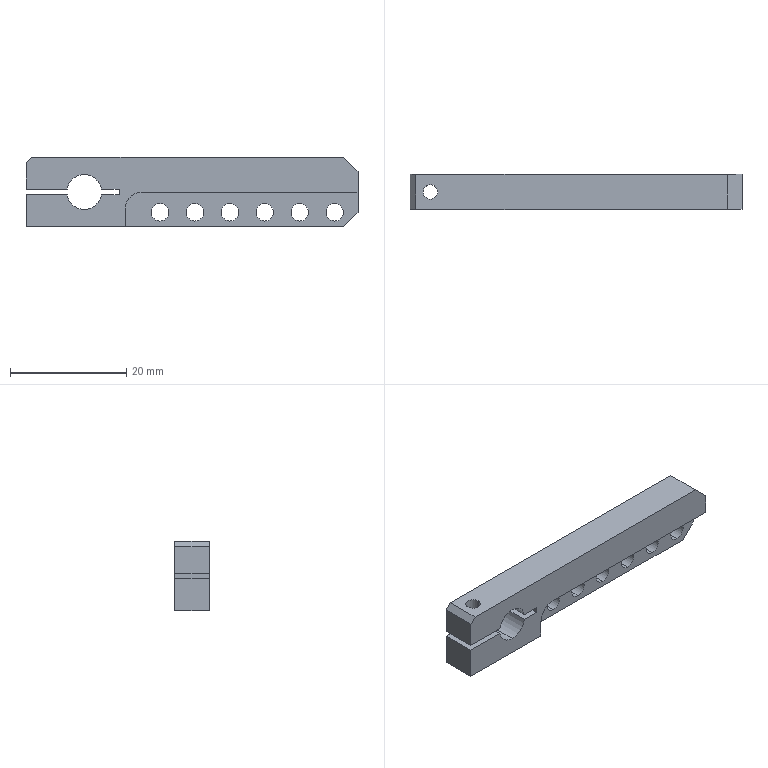Part | SolidWorks | features ICE 4, 3DProfileFeature 2, Chamfer 2, HoleWzd 2, Extrusion 1, Fillet 1, LPattern 1 | 1 solid | 38 faces | box 57 x 6 x 12 mm | volume 2922 mm3 | cylinder 20 | plane 18 | commonest cylinder face diameters 3 x12 6 x4 2.5 x2 3.5 x2
STEP:
#1=CARTESIAN_POINT('',(-9.5,6.,-2.));
#2=VERTEX_POINT('',#1);
#3=CARTESIAN_POINT('',(-9.5,6.,-5.));
#4=VERTEX_POINT('',#3);
#5=CARTESIAN_POINT('',(-9.5,6.,-3.5));
#6=DIRECTION('',(0.,-1.,0.));
#7=DIRECTION('',(0.,0.,-1.));
#8=AXIS2_PLACEMENT_3D('',#5,#6,#7);
#9=CIRCLE('',#8,1.5);
#10=EDGE_CURVE('',#2,#4,#9,.T.);
#11=ORIENTED_EDGE('',*,*,#10,.F.);
#12=CARTESIAN_POINT('',(-9.5,3.,-2.));
#13=VERTEX_POINT('',#12);
#14=CARTESIAN_POINT('',(-9.5,0.,-2.));
#15=DIRECTION('',(0.,-1.,0.));
#16=VECTOR('',#15,1000.);
#17=LINE('',#14,#16);
#18=EDGE_CURVE('',#2,#13,#17,.T.);
#19=ORIENTED_EDGE('',*,*,#18,.T.);
#20=CARTESIAN_POINT('',(-9.5,3.,-5.));
#21=VERTEX_POINT('',#20);
#22=CARTESIAN_POINT('',(-9.5,3.,-3.5));
#23=DIRECTION('',(0.,-1.,0.));
#24=DIRECTION('',(0.,0.,-1.));
#25=AXIS2_PLACEMENT_3D('',#22,#23,#24);
#26=CIRCLE('',#25,1.5);
#27=EDGE_CURVE('',#13,#21,#26,.T.);
#28=ORIENTED_EDGE('',*,*,#27,.T.);
#29=CARTESIAN_POINT('',(-9.5,0.,-5.));
#30=DIRECTION('',(0.,-1.,0.));
#31=VECTOR('',#30,1000.);
#32=LINE('',#29,#31);
#33=EDGE_CURVE('',#4,#21,#32,.T.);
#34=ORIENTED_EDGE('',*,*,#33,.F.);
#35=EDGE_LOOP('',(#11,#19,#28,#34));
#36=FACE_OUTER_BOUND('',#35,.T.);
#37=CARTESIAN_POINT('',(-9.5,0.,-3.5));
#38=DIRECTION('',(0.,-1.,0.));
#39=DIRECTION('',(0.,0.,-1.));
#40=AXIS2_PLACEMENT_3D('',#37,#38,#39);
#41=CYLINDRICAL_SURFACE('',#40,1.5);
#42=ADVANCED_FACE('',(#36),#41,.F.);
#43=CARTESIAN_POINT('',(-3.5,6.,-2.));
#44=VERTEX_POINT('',#43);
#45=CARTESIAN_POINT('',(-3.5,6.,-5.));
#46=VERTEX_POINT('',#45);
#47=CARTESIAN_POINT('',(-3.5,6.,-3.5));
#48=DIRECTION('',(0.,-1.,0.));
#49=DIRECTION('',(0.,0.,-1.));
#50=AXIS2_PLACEMENT_3D('',#47,#48,#49);
#51=CIRCLE('',#50,1.5);
#52=EDGE_CURVE('',#44,#46,#51,.T.);
#53=ORIENTED_EDGE('',*,*,#52,.F.);
#54=CARTESIAN_POINT('',(-3.5,3.,-2.));
#55=VERTEX_POINT('',#54);
#56=CARTESIAN_POINT('',(-3.5,0.,-2.));
#57=DIRECTION('',(0.,-1.,0.));
#58=VECTOR('',#57,1000.);
#59=LINE('',#56,#58);
#60=EDGE_CURVE('',#44,#55,#59,.T.);
#61=ORIENTED_EDGE('',*,*,#60,.T.);
#62=CARTESIAN_POINT('',(-3.5,3.,-5.));
#63=VERTEX_POINT('',#62);
#64=CARTESIAN_POINT('',(-3.5,3.,-3.5));
#65=DIRECTION('',(0.,-1.,0.));
#66=DIRECTION('',(0.,0.,-1.));
#67=AXIS2_PLACEMENT_3D('',#64,#65,#66);
#68=CIRCLE('',#67,1.5);
#69=EDGE_CURVE('',#55,#63,#68,.T.);
#70=ORIENTED_EDGE('',*,*,#69,.T.);
#71=CARTESIAN_POINT('',(-3.5,0.,-5.));
#72=DIRECTION('',(0.,-1.,0.));
#73=VECTOR('',#72,1000.);
#74=LINE('',#71,#73);
#75=EDGE_CURVE('',#46,#63,#74,.T.);
#76=ORIENTED_EDGE('',*,*,#75,.F.);
#77=EDGE_LOOP('',(#53,#61,#70,#76));
#78=FACE_OUTER_BOUND('',#77,.T.);
#79=CARTESIAN_POINT('',(-3.5,0.,-3.5));
#80=DIRECTION('',(0.,-1.,0.));
#81=DIRECTION('',(0.,0.,-1.));
#82=AXIS2_PLACEMENT_3D('',#79,#80,#81);
#83=CYLINDRICAL_SURFACE('',#82,1.5);
#84=ADVANCED_FACE('',(#78),#83,.F.);
#85=CARTESIAN_POINT('',(2.5,6.,-2.));
#86=VERTEX_POINT('',#85);
#87=CARTESIAN_POINT('',(2.5,6.,-5.));
#88=VERTEX_POINT('',#87);
#89=CARTESIAN_POINT('',(2.5,6.,-3.5));
#90=DIRECTION('',(0.,-1.,0.));
#91=DIRECTION('',(0.,0.,-1.));
#92=AXIS2_PLACEMENT_3D('',#89,#90,#91);
#93=CIRCLE('',#92,1.5);
#94=EDGE_CURVE('',#86,#88,#93,.T.);
#95=ORIENTED_EDGE('',*,*,#94,.F.);
#96=CARTESIAN_POINT('',(2.5,3.,-2.));
#97=VERTEX_POINT('',#96);
#98=CARTESIAN_POINT('',(2.5,0.,-2.));
#99=DIRECTION('',(0.,-1.,0.));
#100=VECTOR('',#99,1000.);
#101=LINE('',#98,#100);
#102=EDGE_CURVE('',#86,#97,#101,.T.);
#103=ORIENTED_EDGE('',*,*,#102,.T.);
#104=CARTESIAN_POINT('',(2.5,3.,-5.));
#105=VERTEX_POINT('',#104);
#106=CARTESIAN_POINT('',(2.5,3.,-3.5));
#107=DIRECTION('',(0.,-1.,0.));
#108=DIRECTION('',(0.,0.,-1.));
#109=AXIS2_PLACEMENT_3D('',#106,#107,#108);
#110=CIRCLE('',#109,1.5);
#111=EDGE_CURVE('',#97,#105,#110,.T.);
#112=ORIENTED_EDGE('',*,*,#111,.T.);
#113=CARTESIAN_POINT('',(2.5,0.,-5.));
#114=DIRECTION('',(0.,-1.,0.));
#115=VECTOR('',#114,1000.);
#116=LINE('',#113,#115);
#117=EDGE_CURVE('',#88,#105,#116,.T.);
#118=ORIENTED_EDGE('',*,*,#117,.F.);
#119=EDGE_LOOP('',(#95,#103,#112,#118));
#120=FACE_OUTER_BOUND('',#119,.T.);
#121=CARTESIAN_POINT('',(2.5,0.,-3.5));
#122=DIRECTION('',(0.,-1.,0.));
#123=DIRECTION('',(0.,0.,-1.));
#124=AXIS2_PLACEMENT_3D('',#121,#122,#123);
#125=CYLINDRICAL_SURFACE('',#124,1.5);
#126=ADVANCED_FACE('',(#120),#125,.F.);
#127=CARTESIAN_POINT('',(8.5,6.,-2.));
#128=VERTEX_POINT('',#127);
#129=CARTESIAN_POINT('',(8.5,6.,-5.));
#130=VERTEX_POINT('',#129);
#131=CARTESIAN_POINT('',(8.5,6.,-3.5));
#132=DIRECTION('',(0.,-1.,0.));
#133=DIRECTION('',(0.,0.,-1.));
#134=AXIS2_PLACEMENT_3D('',#131,#132,#133);
#135=CIRCLE('',#134,1.5);
#136=EDGE_CURVE('',#128,#130,#135,.T.);
#137=ORIENTED_EDGE('',*,*,#136,.F.);
#138=CARTESIAN_POINT('',(8.5,3.,-2.));
#139=VERTEX_POINT('',#138);
#140=CARTESIAN_POINT('',(8.5,0.,-2.));
#141=DIRECTION('',(0.,-1.,0.));
#142=VECTOR('',#141,1000.);
#143=LINE('',#140,#142);
#144=EDGE_CURVE('',#128,#139,#143,.T.);
#145=ORIENTED_EDGE('',*,*,#144,.T.);
#146=CARTESIAN_POINT('',(8.5,3.,-5.));
#147=VERTEX_POINT('',#146);
#148=CARTESIAN_POINT('',(8.5,3.,-3.5));
#149=DIRECTION('',(0.,-1.,0.));
#150=DIRECTION('',(0.,0.,-1.));
#151=AXIS2_PLACEMENT_3D('',#148,#149,#150);
#152=CIRCLE('',#151,1.5);
#153=EDGE_CURVE('',#139,#147,#152,.T.);
#154=ORIENTED_EDGE('',*,*,#153,.T.);
#155=CARTESIAN_POINT('',(8.5,0.,-5.));
#156=DIRECTION('',(0.,-1.,0.));
#157=VECTOR('',#156,1000.);
#158=LINE('',#155,#157);
#159=EDGE_CURVE('',#130,#147,#158,.T.);
#160=ORIENTED_EDGE('',*,*,#159,.F.);
#161=EDGE_LOOP('',(#137,#145,#154,#160));
#162=FACE_OUTER_BOUND('',#161,.T.);
#163=CARTESIAN_POINT('',(8.5,0.,-3.5));
#164=DIRECTION('',(0.,-1.,0.));
#165=DIRECTION('',(0.,0.,-1.));
#166=AXIS2_PLACEMENT_3D('',#163,#164,#165);
#167=CYLINDRICAL_SURFACE('',#166,1.5);
#168=ADVANCED_FACE('',(#162),#167,.F.);
#169=CARTESIAN_POINT('',(14.5,6.,-2.));
#170=VERTEX_POINT('',#169);
#171=CARTESIAN_POINT('',(14.5,6.,-5.));
#172=VERTEX_POINT('',#171);
#173=CARTESIAN_POINT('',(14.5,6.,-3.5));
#174=DIRECTION('',(0.,-1.,0.));
#175=DIRECTION('',(0.,0.,-1.));
#176=AXIS2_PLACEMENT_3D('',#173,#174,#175);
#177=CIRCLE('',#176,1.5);
#178=EDGE_CURVE('',#170,#172,#177,.T.);
#179=ORIENTED_EDGE('',*,*,#178,.F.);
#180=CARTESIAN_POINT('',(14.5,3.,-2.));
#181=VERTEX_POINT('',#180);
#182=CARTESIAN_POINT('',(14.5,0.,-2.));
#183=DIRECTION('',(0.,-1.,0.));
#184=VECTOR('',#183,1000.);
#185=LINE('',#182,#184);
#186=EDGE_CURVE('',#170,#181,#185,.T.);
#187=ORIENTED_EDGE('',*,*,#186,.T.);
#188=CARTESIAN_POINT('',(14.5,3.,-5.));
#189=VERTEX_POINT('',#188);
#190=CARTESIAN_POINT('',(14.5,3.,-3.5));
#191=DIRECTION('',(0.,-1.,0.));
#192=DIRECTION('',(0.,0.,-1.));
#193=AXIS2_PLACEMENT_3D('',#190,#191,#192);
#194=CIRCLE('',#193,1.5);
#195=EDGE_CURVE('',#181,#189,#194,.T.);
#196=ORIENTED_EDGE('',*,*,#195,.T.);
#197=CARTESIAN_POINT('',(14.5,0.,-5.));
#198=DIRECTION('',(0.,-1.,0.));
#199=VECTOR('',#198,1000.);
#200=LINE('',#197,#199);
#201=EDGE_CURVE('',#172,#189,#200,.T.);
#202=ORIENTED_EDGE('',*,*,#201,.F.);
#203=EDGE_LOOP('',(#179,#187,#196,#202));
#204=FACE_OUTER_BOUND('',#203,.T.);
#205=CARTESIAN_POINT('',(14.5,0.,-3.5));
#206=DIRECTION('',(0.,-1.,0.));
#207=DIRECTION('',(0.,0.,-1.));
#208=AXIS2_PLACEMENT_3D('',#205,#206,#207);
#209=CYLINDRICAL_SURFACE('',#208,1.5);
#210=ADVANCED_FACE('',(#204),#209,.F.);
#211=CARTESIAN_POINT('',(20.5,6.,-2.));
#212=VERTEX_POINT('',#211);
#213=CARTESIAN_POINT('',(20.5,6.,-5.));
#214=VERTEX_POINT('',#213);
#215=CARTESIAN_POINT('',(20.5,6.,-3.5));
#216=DIRECTION('',(0.,-1.,0.));
#217=DIRECTION('',(0.,0.,-1.));
#218=AXIS2_PLACEMENT_3D('',#215,#216,#217);
#219=CIRCLE('',#218,1.5);
#220=EDGE_CURVE('',#212,#214,#219,.T.);
#221=ORIENTED_EDGE('',*,*,#220,.F.);
#222=CARTESIAN_POINT('',(20.5,3.,-2.));
#223=VERTEX_POINT('',#222);
#224=CARTESIAN_POINT('',(20.5,0.,-2.));
#225=DIRECTION('',(0.,-1.,0.));
#226=VECTOR('',#225,1000.);
#227=LINE('',#224,#226);
#228=EDGE_CURVE('',#212,#223,#227,.T.);
#229=ORIENTED_EDGE('',*,*,#228,.T.);
#230=CARTESIAN_POINT('',(20.5,3.,-5.));
#231=VERTEX_POINT('',#230);
#232=CARTESIAN_POINT('',(20.5,3.,-3.5));
#233=DIRECTION('',(0.,-1.,0.));
#234=DIRECTION('',(0.,0.,-1.));
#235=AXIS2_PLACEMENT_3D('',#232,#233,#234);
#236=CIRCLE('',#235,1.5);
#237=EDGE_CURVE('',#223,#231,#236,.T.);
#238=ORIENTED_EDGE('',*,*,#237,.T.);
#239=CARTESIAN_POINT('',(20.5,0.,-5.));
#240=DIRECTION('',(0.,-1.,0.));
#241=VECTOR('',#240,1000.);
#242=LINE('',#239,#241);
#243=EDGE_CURVE('',#214,#231,#242,.T.);
#244=ORIENTED_EDGE('',*,*,#243,.F.);
#245=EDGE_LOOP('',(#221,#229,#238,#244));
#246=FACE_OUTER_BOUND('',#245,.T.);
#247=CARTESIAN_POINT('',(20.5,0.,-3.5));
#248=DIRECTION('',(0.,-1.,0.));
#249=DIRECTION('',(0.,0.,-1.));
#250=AXIS2_PLACEMENT_3D('',#247,#248,#249);
#251=CYLINDRICAL_SURFACE('',#250,1.5);
#252=ADVANCED_FACE('',(#246),#251,.F.);
#253=CARTESIAN_POINT('',(-27.75,3.,6.));
#254=VERTEX_POINT('',#253);
#255=CARTESIAN_POINT('',(-30.25,3.,6.));
#256=VERTEX_POINT('',#255);
#257=CARTESIAN_POINT('',(-29.,3.,6.));
#258=DIRECTION('',(0.,0.,-1.));
#259=DIRECTION('',(-1.,0.,0.));
#260=AXIS2_PLACEMENT_3D('',#257,#258,#259);
#261=CIRCLE('',#260,1.25);
#262=EDGE_CURVE('',#254,#256,#261,.T.);
#263=ORIENTED_EDGE('',*,*,#262,.F.);
#264=CARTESIAN_POINT('',(-27.75,3.,0.5));
#265=VERTEX_POINT('',#264);
#266=CARTESIAN_POINT('',(-27.75,3.,0.5));
#267=DIRECTION('',(0.,0.,-1.));
#268=VECTOR('',#267,1000.);
#269=LINE('',#266,#268);
#270=EDGE_CURVE('',#254,#265,#269,.T.);
#271=ORIENTED_EDGE('',*,*,#270,.T.);
#272=CARTESIAN_POINT('',(-30.25,3.,0.5));
#273=VERTEX_POINT('',#272);
#274=CARTESIAN_POINT('',(-29.,3.,0.5));
#275=DIRECTION('',(0.,0.,-1.));
#276=DIRECTION('',(-1.,0.,0.));
#277=AXIS2_PLACEMENT_3D('',#274,#275,#276);
#278=CIRCLE('',#277,1.25);
#279=EDGE_CURVE('',#265,#273,#278,.T.);
#280=ORIENTED_EDGE('',*,*,#279,.T.);
#281=CARTESIAN_POINT('',(-30.25,3.,0.5));
#282=DIRECTION('',(0.,0.,-1.));
#283=VECTOR('',#282,1000.);
#284=LINE('',#281,#283);
#285=EDGE_CURVE('',#256,#273,#284,.T.);
#286=ORIENTED_EDGE('',*,*,#285,.F.);
#287=EDGE_LOOP('',(#263,#271,#280,#286));
#288=FACE_OUTER_BOUND('',#287,.T.);
#289=CARTESIAN_POINT('',(-29.,3.,0.5));
#290=DIRECTION('',(0.,0.,-1.));
#291=DIRECTION('',(-1.,0.,0.));
#292=AXIS2_PLACEMENT_3D('',#289,#290,#291);
#293=CYLINDRICAL_SURFACE('',#292,1.25);
#294=ADVANCED_FACE('',(#288),#293,.F.);
#295=CARTESIAN_POINT('',(-27.25,3.,-0.5));
#296=VERTEX_POINT('',#295);
#297=CARTESIAN_POINT('',(-30.75,3.,-0.5));
#298=VERTEX_POINT('',#297);
#299=CARTESIAN_POINT('',(-29.,3.,-0.5));
#300=DIRECTION('',(0.,0.,-1.));
#301=DIRECTION('',(-1.,0.,0.));
#302=AXIS2_PLACEMENT_3D('',#299,#300,#301);
#303=CIRCLE('',#302,1.75);
#304=EDGE_CURVE('',#296,#298,#303,.T.);
#305=ORIENTED_EDGE('',*,*,#304,.F.);
#306=CARTESIAN_POINT('',(-27.25,3.,-6.));
#307=VERTEX_POINT('',#306);
#308=CARTESIAN_POINT('',(-27.25,3.,0.));
#309=DIRECTION('',(0.,0.,-1.));
#310=VECTOR('',#309,1000.);
#311=LINE('',#308,#310);
#312=EDGE_CURVE('',#296,#307,#311,.T.);
#313=ORIENTED_EDGE('',*,*,#312,.T.);
#314=CARTESIAN_POINT('',(-30.75,3.,-6.));
#315=VERTEX_POINT('',#314);
#316=CARTESIAN_POINT('',(-29.,3.,-6.));
#317=DIRECTION('',(0.,0.,-1.));
#318=DIRECTION('',(-1.,0.,0.));
#319=AXIS2_PLACEMENT_3D('',#316,#317,#318);
#320=CIRCLE('',#319,1.75);
#321=EDGE_CURVE('',#307,#315,#320,.T.);
#322=ORIENTED_EDGE('',*,*,#321,.T.);
#323=CARTESIAN_POINT('',(-30.75,3.,0.));
#324=DIRECTION('',(0.,0.,-1.));
#325=VECTOR('',#324,1000.);
#326=LINE('',#323,#325);
#327=EDGE_CURVE('',#298,#315,#326,.T.);
#328=ORIENTED_EDGE('',*,*,#327,.F.);
#329=EDGE_LOOP('',(#305,#313,#322,#328));
#330=FACE_OUTER_BOUND('',#329,.T.);
#331=CARTESIAN_POINT('',(-29.,3.,0.));
#332=DIRECTION('',(0.,0.,-1.));
#333=DIRECTION('',(-1.,0.,0.));
#334=AXIS2_PLACEMENT_3D('',#331,#332,#333);
#335=CYLINDRICAL_SURFACE('',#334,1.75);
#336=ADVANCED_FACE('',(#330),#335,.F.);
#337=CARTESIAN_POINT('',(-19.542,6.,-0.5));
#338=VERTEX_POINT('',#337);
#339=CARTESIAN_POINT('',(-22.5,6.,-3.));
#340=VERTEX_POINT('',#339);
#341=CARTESIAN_POINT('',(-22.5,6.,0.));
#342=DIRECTION('',(0.,1.,0.));
#343=DIRECTION('',(0.,0.,1.));
#344=AXIS2_PLACEMENT_3D('',#341,#342,#343);
#345=CIRCLE('',#344,3.);
#346=EDGE_CURVE('',#338,#340,#345,.T.);
#347=ORIENTED_EDGE('',*,*,#346,.T.);
#348=CARTESIAN_POINT('',(-22.5,0.,-3.));
#349=VERTEX_POINT('',#348);
#350=CARTESIAN_POINT('',(-22.5,6.,-3.));
#351=DIRECTION('',(0.,-1.,0.));
#352=VECTOR('',#351,1000.);
#353=LINE('',#350,#352);
#354=EDGE_CURVE('',#340,#349,#353,.T.);
#355=ORIENTED_EDGE('',*,*,#354,.T.);
#356=CARTESIAN_POINT('',(-19.542,0.,-0.5));
#357=VERTEX_POINT('',#356);
#358=CARTESIAN_POINT('',(-22.5,0.,0.));
#359=DIRECTION('',(0.,1.,0.));
#360=DIRECTION('',(0.,0.,1.));
#361=AXIS2_PLACEMENT_3D('',#358,#359,#360);
#362=CIRCLE('',#361,3.);
#363=EDGE_CURVE('',#357,#349,#362,.T.);
#364=ORIENTED_EDGE('',*,*,#363,.F.);
#365=CARTESIAN_POINT('',(-19.542,6.,-0.5));
#366=DIRECTION('',(0.,-1.,0.));
#367=VECTOR('',#366,1000.);
#368=LINE('',#365,#367);
#369=EDGE_CURVE('',#338,#357,#368,.T.);
#370=ORIENTED_EDGE('',*,*,#369,.F.);
#371=EDGE_LOOP('',(#347,#355,#364,#370));
#372=FACE_OUTER_BOUND('',#371,.T.);
#373=CARTESIAN_POINT('',(-22.5,6.,0.));
#374=DIRECTION('',(0.,-1.,0.));
#375=DIRECTION('',(0.,0.,-1.));
#376=AXIS2_PLACEMENT_3D('',#373,#374,#375);
#377=CYLINDRICAL_SURFACE('',#376,3.);
#378=ADVANCED_FACE('',(#372),#377,.F.);
#379=CARTESIAN_POINT('',(24.5,6.,-3.5));
#380=VERTEX_POINT('',#379);
#381=CARTESIAN_POINT('',(24.5,6.,3.5));
#382=VERTEX_POINT('',#381);
#383=CARTESIAN_POINT('',(24.5,6.,0.));
#384=DIRECTION('',(0.,0.,1.));
#385=VECTOR('',#384,1000.);
#386=LINE('',#383,#385);
#387=EDGE_CURVE('',#380,#382,#386,.T.);
#388=ORIENTED_EDGE('',*,*,#387,.F.);
#389=CARTESIAN_POINT('',(22.,6.,-6.));
#390=VERTEX_POINT('',#389);
#391=CARTESIAN_POINT('',(14.,6.,-14.));
#392=DIRECTION('',(-0.7071,0.,-0.7071));
#393=VECTOR('',#392,1000.);
#394=LINE('',#391,#393);
#395=EDGE_CURVE('',#380,#390,#394,.T.);
#396=ORIENTED_EDGE('',*,*,#395,.T.);
#397=CARTESIAN_POINT('',(-32.5,6.,-6.));
#398=VERTEX_POINT('',#397);
#399=CARTESIAN_POINT('',(-32.5,6.,-6.));
#400=DIRECTION('',(-1.,0.,0.));
#401=VECTOR('',#400,1000.);
#402=LINE('',#399,#401);
#403=EDGE_CURVE('',#390,#398,#402,.T.);
#404=ORIENTED_EDGE('',*,*,#403,.T.);
#405=CARTESIAN_POINT('',(-32.5,6.,-0.5));
#406=VERTEX_POINT('',#405);
#407=CARTESIAN_POINT('',(-32.5,6.,-6.));
#408=DIRECTION('',(0.,0.,1.));
#409=VECTOR('',#408,1000.);
#410=LINE('',#407,#409);
#411=EDGE_CURVE('',#398,#406,#410,.T.);
#412=ORIENTED_EDGE('',*,*,#411,.T.);
#413=CARTESIAN_POINT('',(-25.458,6.,-0.5));
#414=VERTEX_POINT('',#413);
#415=CARTESIAN_POINT('',(-48.5,6.,-0.5));
#416=DIRECTION('',(1.,0.,0.));
#417=VECTOR('',#416,1000.);
#418=LINE('',#415,#417);
#419=EDGE_CURVE('',#406,#414,#418,.T.);
#420=ORIENTED_EDGE('',*,*,#419,.T.);
#421=CARTESIAN_POINT('',(-22.5,6.,0.));
#422=DIRECTION('',(0.,1.,0.));
#423=DIRECTION('',(0.,0.,1.));
#424=AXIS2_PLACEMENT_3D('',#421,#422,#423);
#425=CIRCLE('',#424,3.);
#426=EDGE_CURVE('',#340,#414,#425,.T.);
#427=ORIENTED_EDGE('',*,*,#426,.F.);
#428=ORIENTED_EDGE('',*,*,#346,.F.);
#429=CARTESIAN_POINT('',(-16.5,6.,-0.5));
#430=VERTEX_POINT('',#429);
#431=CARTESIAN_POINT('',(-48.5,6.,-0.5));
#432=DIRECTION('',(1.,0.,0.));
#433=VECTOR('',#432,1000.);
#434=LINE('',#431,#433);
#435=EDGE_CURVE('',#338,#430,#434,.T.);
#436=ORIENTED_EDGE('',*,*,#435,.T.);
#437=CARTESIAN_POINT('',(-16.5,6.,0.5));
#438=VERTEX_POINT('',#437);
#439=CARTESIAN_POINT('',(-16.5,6.,0.5));
#440=DIRECTION('',(0.,0.,1.));
#441=VECTOR('',#440,1000.);
#442=LINE('',#439,#441);
#443=EDGE_CURVE('',#430,#438,#442,.T.);
#444=ORIENTED_EDGE('',*,*,#443,.T.);
#445=CARTESIAN_POINT('',(-19.542,6.,0.5));
#446=VERTEX_POINT('',#445);
#447=CARTESIAN_POINT('',(-48.5,6.,0.5));
#448=DIRECTION('',(-1.,0.,0.));
#449=VECTOR('',#448,1000.);
#450=LINE('',#447,#449);
#451=EDGE_CURVE('',#438,#446,#450,.T.);
#452=ORIENTED_EDGE('',*,*,#451,.T.);
#453=CARTESIAN_POINT('',(-25.458,6.,0.5));
#454=VERTEX_POINT('',#453);
#455=CARTESIAN_POINT('',(-22.5,6.,0.));
#456=DIRECTION('',(0.,1.,0.));
#457=DIRECTION('',(0.,0.,1.));
#458=AXIS2_PLACEMENT_3D('',#455,#456,#457);
#459=CIRCLE('',#458,3.);
#460=EDGE_CURVE('',#454,#446,#459,.T.);
#461=ORIENTED_EDGE('',*,*,#460,.F.);
#462=CARTESIAN_POINT('',(-32.5,6.,0.5));
#463=VERTEX_POINT('',#462);
#464=CARTESIAN_POINT('',(-48.5,6.,0.5));
#465=DIRECTION('',(-1.,0.,0.));
#466=VECTOR('',#465,1000.);
#467=LINE('',#464,#466);
#468=EDGE_CURVE('',#454,#463,#467,.T.);
#469=ORIENTED_EDGE('',*,*,#468,.T.);
#470=CARTESIAN_POINT('',(-32.5,6.,5.));
#471=VERTEX_POINT('',#470);
#472=CARTESIAN_POINT('',(-32.5,6.,-6.));
#473=DIRECTION('',(0.,0.,1.));
#474=VECTOR('',#473,1000.);
#475=LINE('',#472,#474);
#476=EDGE_CURVE('',#463,#471,#475,.T.);
#477=ORIENTED_EDGE('',*,*,#476,.T.);
#478=CARTESIAN_POINT('',(-31.5,6.,6.));
#479=VERTEX_POINT('',#478);
#480=CARTESIAN_POINT('',(-18.75,6.,18.75));
#481=DIRECTION('',(0.7071,0.,0.7071));
#482=VECTOR('',#481,1000.);
#483=LINE('',#480,#482);
#484=EDGE_CURVE('',#471,#479,#483,.T.);
#485=ORIENTED_EDGE('',*,*,#484,.T.);
#486=CARTESIAN_POINT('',(22.,6.,6.));
#487=VERTEX_POINT('',#486);
#488=CARTESIAN_POINT('',(-32.5,6.,6.));
#489=DIRECTION('',(1.,0.,0.));
#490=VECTOR('',#489,1000.);
#491=LINE('',#488,#490);
#492=EDGE_CURVE('',#479,#487,#491,.T.);
#493=ORIENTED_EDGE('',*,*,#492,.T.);
#494=CARTESIAN_POINT('',(14.,6.,14.));
#495=DIRECTION('',(0.7071,0.,-0.7071));
#496=VECTOR('',#495,1000.);
#497=LINE('',#494,#496);
#498=EDGE_CURVE('',#487,#382,#497,.T.);
#499=ORIENTED_EDGE('',*,*,#498,.T.);
#500=EDGE_LOOP('',(#388,#396,#404,#412,#420,#427,#428,#436,#444,#452,#461,#469,#477,#485,#493,#499));
#501=FACE_OUTER_BOUND('',#500,.T.);
#502=CARTESIAN_POINT('',(-3.5,6.,-3.5));
#503=DIRECTION('',(0.,-1.,0.));
#504=DIRECTION('',(0.,0.,-1.));
#505=AXIS2_PLACEMENT_3D('',#502,#503,#504);
#506=CIRCLE('',#505,1.5);
#507=EDGE_CURVE('',#46,#44,#506,.T.);
#508=ORIENTED_EDGE('',*,*,#507,.T.);
#509=ORIENTED_EDGE('',*,*,#52,.T.);
#510=EDGE_LOOP('',(#508,#509));
#511=FACE_BOUND('',#510,.T.);
#512=CARTESIAN_POINT('',(2.5,6.,-3.5));
#513=DIRECTION('',(0.,-1.,0.));
#514=DIRECTION('',(0.,0.,-1.));
#515=AXIS2_PLACEMENT_3D('',#512,#513,#514);
#516=CIRCLE('',#515,1.5);
#517=EDGE_CURVE('',#88,#86,#516,.T.);
#518=ORIENTED_EDGE('',*,*,#517,.T.);
#519=ORIENTED_EDGE('',*,*,#94,.T.);
#520=EDGE_LOOP('',(#518,#519));
#521=FACE_BOUND('',#520,.T.);
#522=CARTESIAN_POINT('',(8.5,6.,-3.5));
#523=DIRECTION('',(0.,-1.,0.));
#524=DIRECTION('',(0.,0.,-1.));
#525=AXIS2_PLACEMENT_3D('',#522,#523,#524);
#526=CIRCLE('',#525,1.5);
#527=EDGE_CURVE('',#130,#128,#526,.T.);
#528=ORIENTED_EDGE('',*,*,#527,.T.);
#529=ORIENTED_EDGE('',*,*,#136,.T.);
#530=EDGE_LOOP('',(#528,#529));
#531=FACE_BOUND('',#530,.T.);
#532=CARTESIAN_POINT('',(14.5,6.,-3.5));
#533=DIRECTION('',(0.,-1.,0.));
#534=DIRECTION('',(0.,0.,-1.));
#535=AXIS2_PLACEMENT_3D('',#532,#533,#534);
#536=CIRCLE('',#535,1.5);
#537=EDGE_CURVE('',#172,#170,#536,.T.);
#538=ORIENTED_EDGE('',*,*,#537,.T.);
#539=ORIENTED_EDGE('',*,*,#178,.T.);
#540=EDGE_LOOP('',(#538,#539));
#541=FACE_BOUND('',#540,.T.);
#542=CARTESIAN_POINT('',(20.5,6.,-3.5));
#543=DIRECTION('',(0.,-1.,0.));
#544=DIRECTION('',(0.,0.,-1.));
#545=AXIS2_PLACEMENT_3D('',#542,#543,#544);
#546=CIRCLE('',#545,1.5);
#547=EDGE_CURVE('',#214,#212,#546,.T.);
#548=ORIENTED_EDGE('',*,*,#547,.T.);
#549=ORIENTED_EDGE('',*,*,#220,.T.);
#550=EDGE_LOOP('',(#548,#549));
#551=FACE_BOUND('',#550,.T.);
#552=CARTESIAN_POINT('',(-9.5,6.,-3.5));
#553=DIRECTION('',(0.,-1.,0.));
#554=DIRECTION('',(0.,0.,-1.));
#555=AXIS2_PLACEMENT_3D('',#552,#553,#554);
#556=CIRCLE('',#555,1.5);
#557=EDGE_CURVE('',#4,#2,#556,.T.);
#558=ORIENTED_EDGE('',*,*,#557,.T.);
#559=ORIENTED_EDGE('',*,*,#10,.T.);
#560=EDGE_LOOP('',(#558,#559));
#561=FACE_BOUND('',#560,.T.);
#562=CARTESIAN_POINT('',(0.,6.,0.));
#563=DIRECTION('',(0.,1.,0.));
#564=DIRECTION('',(0.,0.,1.));
#565=AXIS2_PLACEMENT_3D('',#562,#563,#564);
#566=PLANE('',#565);
#567=ADVANCED_FACE('',(#501,#511,#521,#531,#541,#551,#561),#566,.T.);
#568=CARTESIAN_POINT('',(-32.5,0.,-6.));
#569=VERTEX_POINT('',#568);
#570=CARTESIAN_POINT('',(-32.5,0.,-0.5));
#571=VERTEX_POINT('',#570);
#572=CARTESIAN_POINT('',(-32.5,0.,-6.));
#573=DIRECTION('',(0.,0.,1.));
#574=VECTOR('',#573,1000.);
#575=LINE('',#572,#574);
#576=EDGE_CURVE('',#569,#571,#575,.T.);
#577=ORIENTED_EDGE('',*,*,#576,.T.);
#578=CARTESIAN_POINT('',(-32.5,6.,-0.5));
#579=DIRECTION('',(0.,1.,0.));
#580=VECTOR('',#579,1000.);
#581=LINE('',#578,#580);
#582=EDGE_CURVE('',#571,#406,#581,.T.);
#583=ORIENTED_EDGE('',*,*,#582,.T.);
#584=ORIENTED_EDGE('',*,*,#411,.F.);
#585=CARTESIAN_POINT('',(-32.5,6.,-6.));
#586=DIRECTION('',(0.,-1.,0.));
#587=VECTOR('',#586,1000.);
#588=LINE('',#585,#587);
#589=EDGE_CURVE('',#398,#569,#588,.T.);
#590=ORIENTED_EDGE('',*,*,#589,.T.);
#591=EDGE_LOOP('',(#577,#583,#584,#590));
#592=FACE_OUTER_BOUND('',#591,.T.);
#593=CARTESIAN_POINT('',(-32.5,6.,-6.));
#594=DIRECTION('',(1.,0.,0.));
#595=DIRECTION('',(0.,0.,-1.));
#596=AXIS2_PLACEMENT_3D('',#593,#594,#595);
#597=PLANE('',#596);
#598=ADVANCED_FACE('',(#592),#597,.F.);
#599=ORIENTED_EDGE('',*,*,#354,.F.);
#600=ORIENTED_EDGE('',*,*,#426,.T.);
#601=CARTESIAN_POINT('',(-25.458,0.,-0.5));
#602=VERTEX_POINT('',#601);
#603=CARTESIAN_POINT('',(-25.458,6.,-0.5));
#604=DIRECTION('',(0.,1.,0.));
#605=VECTOR('',#604,1000.);
#606=LINE('',#603,#605);
#607=EDGE_CURVE('',#602,#414,#606,.T.);
#608=ORIENTED_EDGE('',*,*,#607,.F.);
#609=CARTESIAN_POINT('',(-22.5,0.,0.));
#610=DIRECTION('',(0.,1.,0.));
#611=DIRECTION('',(0.,0.,1.));
#612=AXIS2_PLACEMENT_3D('',#609,#610,#611);
#613=CIRCLE('',#612,3.);
#614=EDGE_CURVE('',#349,#602,#613,.T.);
#615=ORIENTED_EDGE('',*,*,#614,.F.);
#616=EDGE_LOOP('',(#599,#600,#608,#615));
#617=FACE_OUTER_BOUND('',#616,.T.);
#618=CARTESIAN_POINT('',(-22.5,6.,0.));
#619=DIRECTION('',(0.,-1.,0.));
#620=DIRECTION('',(0.,0.,-1.));
#621=AXIS2_PLACEMENT_3D('',#618,#619,#620);
#622=CYLINDRICAL_SURFACE('',#621,3.);
#623=ADVANCED_FACE('',(#617),#622,.F.);
#624=CARTESIAN_POINT('',(24.5,0.,3.5));
#625=VERTEX_POINT('',#624);
#626=CARTESIAN_POINT('',(24.5,0.,0.));
#627=VERTEX_POINT('',#626);
#628=CARTESIAN_POINT('',(24.5,0.,6.));
#629=DIRECTION('',(0.,0.,-1.));
#630=VECTOR('',#629,1000.);
#631=LINE('',#628,#630);
#632=EDGE_CURVE('',#625,#627,#631,.T.);
#633=ORIENTED_EDGE('',*,*,#632,.F.);
#634=CARTESIAN_POINT('',(22.,0.,6.));
#635=VERTEX_POINT('',#634);
#636=CARTESIAN_POINT('',(24.5,0.,3.5));
#637=DIRECTION('',(-0.7071,0.,0.7071));
#638=VECTOR('',#637,1000.);
#639=LINE('',#636,#638);
#640=EDGE_CURVE('',#625,#635,#639,.T.);
#641=ORIENTED_EDGE('',*,*,#640,.T.);
#642=CARTESIAN_POINT('',(-31.5,0.,6.));
#643=VERTEX_POINT('',#642);
#644=CARTESIAN_POINT('',(-32.5,0.,6.));
#645=DIRECTION('',(1.,0.,0.));
#646=VECTOR('',#645,1000.);
#647=LINE('',#644,#646);
#648=EDGE_CURVE('',#643,#635,#647,.T.);
#649=ORIENTED_EDGE('',*,*,#648,.F.);
#650=CARTESIAN_POINT('',(-32.5,0.,5.));
#651=VERTEX_POINT('',#650);
#652=CARTESIAN_POINT('',(-31.5,0.,6.));
#653=DIRECTION('',(-0.7071,0.,-0.7071));
#654=VECTOR('',#653,1000.);
#655=LINE('',#652,#654);
#656=EDGE_CURVE('',#643,#651,#655,.T.);
#657=ORIENTED_EDGE('',*,*,#656,.T.);
#658=CARTESIAN_POINT('',(-32.5,0.,0.5));
#659=VERTEX_POINT('',#658);
#660=CARTESIAN_POINT('',(-32.5,0.,-6.));
#661=DIRECTION('',(0.,0.,1.));
#662=VECTOR('',#661,1000.);
#663=LINE('',#660,#662);
#664=EDGE_CURVE('',#659,#651,#663,.T.);
#665=ORIENTED_EDGE('',*,*,#664,.F.);
#666=CARTESIAN_POINT('',(-25.458,0.,0.5));
#667=VERTEX_POINT('',#666);
#668=CARTESIAN_POINT('',(-48.5,0.,0.5));
#669=DIRECTION('',(-1.,0.,0.));
#670=VECTOR('',#669,1000.);
#671=LINE('',#668,#670);
#672=EDGE_CURVE('',#667,#659,#671,.T.);
#673=ORIENTED_EDGE('',*,*,#672,.F.);
#674=CARTESIAN_POINT('',(-19.542,0.,0.5));
#675=VERTEX_POINT('',#674);
#676=CARTESIAN_POINT('',(-22.5,0.,0.));
#677=DIRECTION('',(0.,1.,0.));
#678=DIRECTION('',(0.,0.,1.));
#679=AXIS2_PLACEMENT_3D('',#676,#677,#678);
#680=CIRCLE('',#679,3.);
#681=EDGE_CURVE('',#667,#675,#680,.T.);
#682=ORIENTED_EDGE('',*,*,#681,.T.);
#683=CARTESIAN_POINT('',(-16.5,0.,0.5));
#684=VERTEX_POINT('',#683);
#685=CARTESIAN_POINT('',(-48.5,0.,0.5));
#686=DIRECTION('',(-1.,0.,0.));
#687=VECTOR('',#686,1000.);
#688=LINE('',#685,#687);
#689=EDGE_CURVE('',#684,#675,#688,.T.);
#690=ORIENTED_EDGE('',*,*,#689,.F.);
#691=CARTESIAN_POINT('',(-16.5,0.,-0.5));
#692=VERTEX_POINT('',#691);
#693=CARTESIAN_POINT('',(-16.5,0.,0.5));
#694=DIRECTION('',(0.,0.,1.));
#695=VECTOR('',#694,1000.);
#696=LINE('',#693,#695);
#697=EDGE_CURVE('',#692,#684,#696,.T.);
#698=ORIENTED_EDGE('',*,*,#697,.F.);
#699=CARTESIAN_POINT('',(-48.5,0.,-0.5));
#700=DIRECTION('',(1.,0.,0.));
#701=VECTOR('',#700,1000.);
#702=LINE('',#699,#701);
#703=EDGE_CURVE('',#357,#692,#702,.T.);
#704=ORIENTED_EDGE('',*,*,#703,.F.);
#705=ORIENTED_EDGE('',*,*,#363,.T.);
#706=ORIENTED_EDGE('',*,*,#614,.T.);
#707=CARTESIAN_POINT('',(-48.5,0.,-0.5));
#708=DIRECTION('',(1.,0.,0.));
#709=VECTOR('',#708,1000.);
#710=LINE('',#707,#709);
#711=EDGE_CURVE('',#571,#602,#710,.T.);
#712=ORIENTED_EDGE('',*,*,#711,.F.);
#713=ORIENTED_EDGE('',*,*,#576,.F.);
#714=CARTESIAN_POINT('',(-15.5,0.,-6.));
#715=VERTEX_POINT('',#714);
#716=CARTESIAN_POINT('',(-32.5,0.,-6.));
#717=DIRECTION('',(-1.,0.,0.));
#718=VECTOR('',#717,1000.);
#719=LINE('',#716,#718);
#720=EDGE_CURVE('',#715,#569,#719,.T.);
#721=ORIENTED_EDGE('',*,*,#720,.F.);
#722=CARTESIAN_POINT('',(-15.5,0.,-3.));
#723=VERTEX_POINT('',#722);
#724=CARTESIAN_POINT('',(-15.5,0.,-6.));
#725=DIRECTION('',(0.,0.,-1.));
#726=VECTOR('',#725,1000.);
#727=LINE('',#724,#726);
#728=EDGE_CURVE('',#723,#715,#727,.T.);
#729=ORIENTED_EDGE('',*,*,#728,.F.);
#730=CARTESIAN_POINT('',(-12.5,0.,0.));
#731=VERTEX_POINT('',#730);
#732=CARTESIAN_POINT('',(-12.5,0.,-3.));
#733=DIRECTION('',(0.,1.,0.));
#734=DIRECTION('',(0.,0.,1.));
#735=AXIS2_PLACEMENT_3D('',#732,#733,#734);
#736=CIRCLE('',#735,3.);
#737=EDGE_CURVE('',#723,#731,#736,.T.);
#738=ORIENTED_EDGE('',*,*,#737,.T.);
#739=CARTESIAN_POINT('',(32.5,0.,0.));
#740=DIRECTION('',(-1.,0.,0.));
#741=VECTOR('',#740,1000.);
#742=LINE('',#739,#741);
#743=EDGE_CURVE('',#627,#731,#742,.T.);
#744=ORIENTED_EDGE('',*,*,#743,.F.);
#745=EDGE_LOOP('',(#633,#641,#649,#657,#665,#673,#682,#690,#698,#704,#705,#706,#712,#713,#721,#729,#738,#744));
#746=FACE_OUTER_BOUND('',#745,.T.);
#747=CARTESIAN_POINT('',(0.,0.,0.));
#748=DIRECTION('',(0.,1.,0.));
#749=DIRECTION('',(0.,0.,1.));
#750=AXIS2_PLACEMENT_3D('',#747,#748,#749);
#751=PLANE('',#750);
#752=ADVANCED_FACE('',(#746),#751,.F.);
#753=CARTESIAN_POINT('',(-29.,3.,-6.));
#754=DIRECTION('',(0.,0.,-1.));
#755=DIRECTION('',(-1.,0.,0.));
#756=AXIS2_PLACEMENT_3D('',#753,#754,#755);
#757=CIRCLE('',#756,1.75);
#758=EDGE_CURVE('',#315,#307,#757,.T.);
#759=ORIENTED_EDGE('',*,*,#758,.F.);
#760=ORIENTED_EDGE('',*,*,#321,.F.);
#761=EDGE_LOOP('',(#759,#760));
#762=FACE_BOUND('',#761,.T.);
#763=ORIENTED_EDGE('',*,*,#403,.F.);
#764=CARTESIAN_POINT('',(22.,3.,-6.));
#765=VERTEX_POINT('',#764);
#766=CARTESIAN_POINT('',(22.,6.,-6.));
#767=DIRECTION('',(0.,-1.,0.));
#768=VECTOR('',#767,1000.);
#769=LINE('',#766,#768);
#770=EDGE_CURVE('',#390,#765,#769,.T.);
#771=ORIENTED_EDGE('',*,*,#770,.T.);
#772=CARTESIAN_POINT('',(-15.5,3.,-6.));
#773=VERTEX_POINT('',#772);
#774=CARTESIAN_POINT('',(32.5,3.,-6.));
#775=DIRECTION('',(1.,0.,0.));
#776=VECTOR('',#775,1000.);
#777=LINE('',#774,#776);
#778=EDGE_CURVE('',#773,#765,#777,.T.);
#779=ORIENTED_EDGE('',*,*,#778,.F.);
#780=CARTESIAN_POINT('',(-15.5,3.,-6.));
#781=DIRECTION('',(0.,-1.,0.));
#782=VECTOR('',#781,1000.);
#783=LINE('',#780,#782);
#784=EDGE_CURVE('',#773,#715,#783,.T.);
#785=ORIENTED_EDGE('',*,*,#784,.T.);
#786=ORIENTED_EDGE('',*,*,#720,.T.);
#787=ORIENTED_EDGE('',*,*,#589,.F.);
#788=EDGE_LOOP('',(#763,#771,#779,#785,#786,#787));
#789=FACE_OUTER_BOUND('',#788,.T.);
#790=CARTESIAN_POINT('',(-32.5,6.,-6.));
#791=DIRECTION('',(0.,0.,1.));
#792=DIRECTION('',(1.,0.,0.));
#793=AXIS2_PLACEMENT_3D('',#790,#791,#792);
#794=PLANE('',#793);
#795=ADVANCED_FACE('',(#762,#789),#794,.F.);
#796=ORIENTED_EDGE('',*,*,#664,.T.);
#797=CARTESIAN_POINT('',(-32.5,6.,5.));
#798=DIRECTION('',(0.,1.,0.));
#799=VECTOR('',#798,1000.);
#800=LINE('',#797,#799);
#801=EDGE_CURVE('',#651,#471,#800,.T.);
#802=ORIENTED_EDGE('',*,*,#801,.T.);
#803=ORIENTED_EDGE('',*,*,#476,.F.);
#804=CARTESIAN_POINT('',(-32.5,6.,0.5));
#805=DIRECTION('',(0.,-1.,0.));
#806=VECTOR('',#805,1000.);
#807=LINE('',#804,#806);
#808=EDGE_CURVE('',#463,#659,#807,.T.);
#809=ORIENTED_EDGE('',*,*,#808,.T.);
#810=EDGE_LOOP('',(#796,#802,#803,#809));
#811=FACE_OUTER_BOUND('',#810,.T.);
#812=CARTESIAN_POINT('',(-32.5,6.,-6.));
#813=DIRECTION('',(1.,0.,0.));
#814=DIRECTION('',(0.,0.,-1.));
#815=AXIS2_PLACEMENT_3D('',#812,#813,#814);
#816=PLANE('',#815);
#817=ADVANCED_FACE('',(#811),#816,.F.);
#818=CARTESIAN_POINT('',(-29.,3.,6.));
#819=DIRECTION('',(0.,0.,-1.));
#820=DIRECTION('',(-1.,0.,0.));
#821=AXIS2_PLACEMENT_3D('',#818,#819,#820);
#822=CIRCLE('',#821,1.25);
#823=EDGE_CURVE('',#256,#254,#822,.T.);
#824=ORIENTED_EDGE('',*,*,#823,.T.);
#825=ORIENTED_EDGE('',*,*,#262,.T.);
#826=EDGE_LOOP('',(#824,#825));
#827=FACE_BOUND('',#826,.T.);
#828=ORIENTED_EDGE('',*,*,#648,.T.);
#829=CARTESIAN_POINT('',(22.,6.,6.));
#830=DIRECTION('',(0.,1.,0.));
#831=VECTOR('',#830,1000.);
#832=LINE('',#829,#831);
#833=EDGE_CURVE('',#635,#487,#832,.T.);
#834=ORIENTED_EDGE('',*,*,#833,.T.);
#835=ORIENTED_EDGE('',*,*,#492,.F.);
#836=CARTESIAN_POINT('',(-31.5,6.,6.));
#837=DIRECTION('',(0.,-1.,0.));
#838=VECTOR('',#837,1000.);
#839=LINE('',#836,#838);
#840=EDGE_CURVE('',#479,#643,#839,.T.);
#841=ORIENTED_EDGE('',*,*,#840,.T.);
#842=EDGE_LOOP('',(#828,#834,#835,#841));
#843=FACE_OUTER_BOUND('',#842,.T.);
#844=CARTESIAN_POINT('',(-32.5,6.,6.));
#845=DIRECTION('',(0.,0.,-1.));
#846=DIRECTION('',(-1.,0.,0.));
#847=AXIS2_PLACEMENT_3D('',#844,#845,#846);
#848=PLANE('',#847);
#849=ADVANCED_FACE('',(#827,#843),#848,.F.);
#850=CARTESIAN_POINT('',(-25.458,6.,0.5));
#851=DIRECTION('',(0.,-1.,0.));
#852=VECTOR('',#851,1000.);
#853=LINE('',#850,#852);
#854=EDGE_CURVE('',#454,#667,#853,.T.);
#855=ORIENTED_EDGE('',*,*,#854,.F.);
#856=ORIENTED_EDGE('',*,*,#460,.T.);
#857=CARTESIAN_POINT('',(-19.542,6.,0.5));
#858=DIRECTION('',(0.,1.,0.));
#859=VECTOR('',#858,1000.);
#860=LINE('',#857,#859);
#861=EDGE_CURVE('',#675,#446,#860,.T.);
#862=ORIENTED_EDGE('',*,*,#861,.F.);
#863=ORIENTED_EDGE('',*,*,#681,.F.);
#864=EDGE_LOOP('',(#855,#856,#862,#863));
#865=FACE_OUTER_BOUND('',#864,.T.);
#866=CARTESIAN_POINT('',(-22.5,6.,0.));
#867=DIRECTION('',(0.,-1.,0.));
#868=DIRECTION('',(0.,0.,-1.));
#869=AXIS2_PLACEMENT_3D('',#866,#867,#868);
#870=CYLINDRICAL_SURFACE('',#869,3.);
#871=ADVANCED_FACE('',(#865),#870,.F.);
#872=ORIENTED_EDGE('',*,*,#861,.T.);
#873=ORIENTED_EDGE('',*,*,#451,.F.);
#874=CARTESIAN_POINT('',(-16.5,6.,0.5));
#875=DIRECTION('',(0.,-1.,0.));
#876=VECTOR('',#875,1000.);
#877=LINE('',#874,#876);
#878=EDGE_CURVE('',#438,#684,#877,.T.);
#879=ORIENTED_EDGE('',*,*,#878,.T.);
#880=ORIENTED_EDGE('',*,*,#689,.T.);
#881=EDGE_LOOP('',(#872,#873,#879,#880));
#882=FACE_OUTER_BOUND('',#881,.T.);
#883=CARTESIAN_POINT('',(-48.5,6.,0.5));
#884=DIRECTION('',(0.,0.,1.));
#885=DIRECTION('',(1.,0.,0.));
#886=AXIS2_PLACEMENT_3D('',#883,#884,#885);
#887=PLANE('',#886);
#888=ADVANCED_FACE('',(#882),#887,.F.);
#889=ORIENTED_EDGE('',*,*,#369,.T.);
#890=ORIENTED_EDGE('',*,*,#703,.T.);
#891=CARTESIAN_POINT('',(-16.5,6.,-0.5));
#892=DIRECTION('',(0.,-1.,0.));
#893=VECTOR('',#892,1000.);
#894=LINE('',#891,#893);
#895=EDGE_CURVE('',#430,#692,#894,.T.);
#896=ORIENTED_EDGE('',*,*,#895,.F.);
#897=ORIENTED_EDGE('',*,*,#435,.F.);
#898=EDGE_LOOP('',(#889,#890,#896,#897));
#899=FACE_OUTER_BOUND('',#898,.T.);
#900=CARTESIAN_POINT('',(-48.5,6.,-0.5));
#901=DIRECTION('',(0.,0.,-1.));
#902=DIRECTION('',(-1.,0.,0.));
#903=AXIS2_PLACEMENT_3D('',#900,#901,#902);
#904=PLANE('',#903);
#905=ADVANCED_FACE('',(#899),#904,.F.);
#906=ORIENTED_EDGE('',*,*,#697,.T.);
#907=ORIENTED_EDGE('',*,*,#878,.F.);
#908=ORIENTED_EDGE('',*,*,#443,.F.);
#909=ORIENTED_EDGE('',*,*,#895,.T.);
#910=EDGE_LOOP('',(#906,#907,#908,#909));
#911=FACE_OUTER_BOUND('',#910,.T.);
#912=CARTESIAN_POINT('',(-16.5,6.,0.5));
#913=DIRECTION('',(1.,0.,0.));
#914=DIRECTION('',(0.,0.,-1.));
#915=AXIS2_PLACEMENT_3D('',#912,#913,#914);
#916=PLANE('',#915);
#917=ADVANCED_FACE('',(#911),#916,.F.);
#918=CARTESIAN_POINT('',(-29.,3.,0.5));
#919=DIRECTION('',(0.,0.,-1.));
#920=DIRECTION('',(-1.,0.,0.));
#921=AXIS2_PLACEMENT_3D('',#918,#919,#920);
#922=CIRCLE('',#921,1.25);
#923=EDGE_CURVE('',#273,#265,#922,.T.);
#924=ORIENTED_EDGE('',*,*,#923,.F.);
#925=ORIENTED_EDGE('',*,*,#279,.F.);
#926=EDGE_LOOP('',(#924,#925));
#927=FACE_BOUND('',#926,.T.);
#928=ORIENTED_EDGE('',*,*,#468,.F.);
#929=ORIENTED_EDGE('',*,*,#854,.T.);
#930=ORIENTED_EDGE('',*,*,#672,.T.);
#931=ORIENTED_EDGE('',*,*,#808,.F.);
#932=EDGE_LOOP('',(#928,#929,#930,#931));
#933=FACE_OUTER_BOUND('',#932,.T.);
#934=CARTESIAN_POINT('',(-48.5,6.,0.5));
#935=DIRECTION('',(0.,0.,1.));
#936=DIRECTION('',(1.,0.,0.));
#937=AXIS2_PLACEMENT_3D('',#934,#935,#936);
#938=PLANE('',#937);
#939=ADVANCED_FACE('',(#927,#933),#938,.F.);
#940=CARTESIAN_POINT('',(-29.,3.,-0.5));
#941=DIRECTION('',(0.,0.,-1.));
#942=DIRECTION('',(-1.,0.,0.));
#943=AXIS2_PLACEMENT_3D('',#940,#941,#942);
#944=CIRCLE('',#943,1.75);
#945=EDGE_CURVE('',#298,#296,#944,.T.);
#946=ORIENTED_EDGE('',*,*,#945,.T.);
#947=ORIENTED_EDGE('',*,*,#304,.T.);
#948=EDGE_LOOP('',(#946,#947));
#949=FACE_BOUND('',#948,.T.);
#950=ORIENTED_EDGE('',*,*,#711,.T.);
#951=ORIENTED_EDGE('',*,*,#607,.T.);
#952=ORIENTED_EDGE('',*,*,#419,.F.);
#953=ORIENTED_EDGE('',*,*,#582,.F.);
#954=EDGE_LOOP('',(#950,#951,#952,#953));
#955=FACE_OUTER_BOUND('',#954,.T.);
#956=CARTESIAN_POINT('',(-48.5,6.,-0.5));
#957=DIRECTION('',(0.,0.,-1.));
#958=DIRECTION('',(-1.,0.,0.));
#959=AXIS2_PLACEMENT_3D('',#956,#957,#958);
#960=PLANE('',#959);
#961=ADVANCED_FACE('',(#949,#955),#960,.F.);
#962=ORIENTED_EDGE('',*,*,#312,.F.);
#963=ORIENTED_EDGE('',*,*,#945,.F.);
#964=ORIENTED_EDGE('',*,*,#327,.T.);
#965=ORIENTED_EDGE('',*,*,#758,.T.);
#966=EDGE_LOOP('',(#962,#963,#964,#965));
#967=FACE_OUTER_BOUND('',#966,.T.);
#968=CARTESIAN_POINT('',(-29.,3.,0.));
#969=DIRECTION('',(0.,0.,-1.));
#970=DIRECTION('',(-1.,0.,0.));
#971=AXIS2_PLACEMENT_3D('',#968,#969,#970);
#972=CYLINDRICAL_SURFACE('',#971,1.75);
#973=ADVANCED_FACE('',(#967),#972,.F.);
#974=ORIENTED_EDGE('',*,*,#270,.F.);
#975=ORIENTED_EDGE('',*,*,#823,.F.);
#976=ORIENTED_EDGE('',*,*,#285,.T.);
#977=ORIENTED_EDGE('',*,*,#923,.T.);
#978=EDGE_LOOP('',(#974,#975,#976,#977));
#979=FACE_OUTER_BOUND('',#978,.T.);
#980=CARTESIAN_POINT('',(-29.,3.,0.5));
#981=DIRECTION('',(0.,0.,-1.));
#982=DIRECTION('',(-1.,0.,0.));
#983=AXIS2_PLACEMENT_3D('',#980,#981,#982);
#984=CYLINDRICAL_SURFACE('',#983,1.25);
#985=ADVANCED_FACE('',(#979),#984,.F.);
#986=CARTESIAN_POINT('',(-15.5,3.,-3.));
#987=VERTEX_POINT('',#986);
#988=CARTESIAN_POINT('',(-15.5,3.,-6.));
#989=DIRECTION('',(0.,0.,-1.));
#990=VECTOR('',#989,1000.);
#991=LINE('',#988,#990);
#992=EDGE_CURVE('',#987,#773,#991,.T.);
#993=ORIENTED_EDGE('',*,*,#992,.F.);
#994=CARTESIAN_POINT('',(-15.5,0.,-3.));
#995=DIRECTION('',(0.,-1.,0.));
#996=VECTOR('',#995,1000.);
#997=LINE('',#994,#996);
#998=EDGE_CURVE('',#987,#723,#997,.T.);
#999=ORIENTED_EDGE('',*,*,#998,.T.);
#1000=ORIENTED_EDGE('',*,*,#728,.T.);
#1001=ORIENTED_EDGE('',*,*,#784,.F.);
#1002=EDGE_LOOP('',(#993,#999,#1000,#1001));
#1003=FACE_OUTER_BOUND('',#1002,.T.);
#1004=CARTESIAN_POINT('',(-15.5,3.,-6.));
#1005=DIRECTION('',(-1.,0.,0.));
#1006=DIRECTION('',(0.,0.,1.));
#1007=AXIS2_PLACEMENT_3D('',#1004,#1005,#1006);
#1008=PLANE('',#1007);
#1009=ADVANCED_FACE('',(#1003),#1008,.F.);
#1010=CARTESIAN_POINT('',(24.5,3.,0.));
#1011=VERTEX_POINT('',#1010);
#1012=CARTESIAN_POINT('',(-12.5,3.,0.));
#1013=VERTEX_POINT('',#1012);
#1014=CARTESIAN_POINT('',(32.5,3.,0.));
#1015=DIRECTION('',(-1.,0.,0.));
#1016=VECTOR('',#1015,1000.);
#1017=LINE('',#1014,#1016);
#1018=EDGE_CURVE('',#1011,#1013,#1017,.T.);
#1019=ORIENTED_EDGE('',*,*,#1018,.F.);
#1020=CARTESIAN_POINT('',(24.5,3.,0.));
#1021=DIRECTION('',(0.,-1.,0.));
#1022=VECTOR('',#1021,1000.);
#1023=LINE('',#1020,#1022);
#1024=EDGE_CURVE('',#1011,#627,#1023,.T.);
#1025=ORIENTED_EDGE('',*,*,#1024,.T.);
#1026=ORIENTED_EDGE('',*,*,#743,.T.);
#1027=CARTESIAN_POINT('',(-12.5,3.,0.));
#1028=DIRECTION('',(0.,1.,0.));
#1029=VECTOR('',#1028,1000.);
#1030=LINE('',#1027,#1029);
#1031=EDGE_CURVE('',#731,#1013,#1030,.T.);
#1032=ORIENTED_EDGE('',*,*,#1031,.T.);
#1033=EDGE_LOOP('',(#1019,#1025,#1026,#1032));
#1034=FACE_OUTER_BOUND('',#1033,.T.);
#1035=CARTESIAN_POINT('',(32.5,3.,0.));
#1036=DIRECTION('',(0.,0.,1.));
#1037=DIRECTION('',(1.,0.,0.));
#1038=AXIS2_PLACEMENT_3D('',#1035,#1036,#1037);
#1039=PLANE('',#1038);
#1040=ADVANCED_FACE('',(#1034),#1039,.F.);
#1041=ORIENTED_EDGE('',*,*,#778,.T.);
#1042=CARTESIAN_POINT('',(24.5,3.,-3.5));
#1043=VERTEX_POINT('',#1042);
#1044=CARTESIAN_POINT('',(14.,3.,-14.));
#1045=DIRECTION('',(0.7071,0.,0.7071));
#1046=VECTOR('',#1045,1000.);
#1047=LINE('',#1044,#1046);
#1048=EDGE_CURVE('',#765,#1043,#1047,.T.);
#1049=ORIENTED_EDGE('',*,*,#1048,.T.);
#1050=CARTESIAN_POINT('',(24.5,3.,0.));
#1051=DIRECTION('',(0.,0.,-1.));
#1052=VECTOR('',#1051,1000.);
#1053=LINE('',#1050,#1052);
#1054=EDGE_CURVE('',#1011,#1043,#1053,.T.);
#1055=ORIENTED_EDGE('',*,*,#1054,.F.);
#1056=ORIENTED_EDGE('',*,*,#1018,.T.);
#1057=CARTESIAN_POINT('',(-12.5,3.,-3.));
#1058=DIRECTION('',(0.,-1.,0.));
#1059=DIRECTION('',(0.,0.,-1.));
#1060=AXIS2_PLACEMENT_3D('',#1057,#1058,#1059);
#1061=CIRCLE('',#1060,3.);
#1062=EDGE_CURVE('',#1013,#987,#1061,.T.);
#1063=ORIENTED_EDGE('',*,*,#1062,.T.);
#1064=ORIENTED_EDGE('',*,*,#992,.T.);
#1065=EDGE_LOOP('',(#1041,#1049,#1055,#1056,#1063,#1064));
#1066=FACE_OUTER_BOUND('',#1065,.T.);
#1067=CARTESIAN_POINT('',(-9.5,3.,-3.5));
#1068=DIRECTION('',(0.,-1.,0.));
#1069=DIRECTION('',(0.,0.,-1.));
#1070=AXIS2_PLACEMENT_3D('',#1067,#1068,#1069);
#1071=CIRCLE('',#1070,1.5);
#1072=EDGE_CURVE('',#21,#13,#1071,.T.);
#1073=ORIENTED_EDGE('',*,*,#1072,.F.);
#1074=ORIENTED_EDGE('',*,*,#27,.F.);
#1075=EDGE_LOOP('',(#1073,#1074));
#1076=FACE_BOUND('',#1075,.T.);
#1077=CARTESIAN_POINT('',(-3.5,3.,-3.5));
#1078=DIRECTION('',(0.,-1.,0.));
#1079=DIRECTION('',(0.,0.,-1.));
#1080=AXIS2_PLACEMENT_3D('',#1077,#1078,#1079);
#1081=CIRCLE('',#1080,1.5);
#1082=EDGE_CURVE('',#63,#55,#1081,.T.);
#1083=ORIENTED_EDGE('',*,*,#1082,.F.);
#1084=ORIENTED_EDGE('',*,*,#69,.F.);
#1085=EDGE_LOOP('',(#1083,#1084));
#1086=FACE_BOUND('',#1085,.T.);
#1087=CARTESIAN_POINT('',(2.5,3.,-3.5));
#1088=DIRECTION('',(0.,-1.,0.));
#1089=DIRECTION('',(0.,0.,-1.));
#1090=AXIS2_PLACEMENT_3D('',#1087,#1088,#1089);
#1091=CIRCLE('',#1090,1.5);
#1092=EDGE_CURVE('',#105,#97,#1091,.T.);
#1093=ORIENTED_EDGE('',*,*,#1092,.F.);
#1094=ORIENTED_EDGE('',*,*,#111,.F.);
#1095=EDGE_LOOP('',(#1093,#1094));
#1096=FACE_BOUND('',#1095,.T.);
#1097=CARTESIAN_POINT('',(8.5,3.,-3.5));
#1098=DIRECTION('',(0.,-1.,0.));
#1099=DIRECTION('',(0.,0.,-1.));
#1100=AXIS2_PLACEMENT_3D('',#1097,#1098,#1099);
#1101=CIRCLE('',#1100,1.5);
#1102=EDGE_CURVE('',#147,#139,#1101,.T.);
#1103=ORIENTED_EDGE('',*,*,#1102,.F.);
#1104=ORIENTED_EDGE('',*,*,#153,.F.);
#1105=EDGE_LOOP('',(#1103,#1104));
#1106=FACE_BOUND('',#1105,.T.);
#1107=CARTESIAN_POINT('',(14.5,3.,-3.5));
#1108=DIRECTION('',(0.,-1.,0.));
#1109=DIRECTION('',(0.,0.,-1.));
#1110=AXIS2_PLACEMENT_3D('',#1107,#1108,#1109);
#1111=CIRCLE('',#1110,1.5);
#1112=EDGE_CURVE('',#189,#181,#1111,.T.);
#1113=ORIENTED_EDGE('',*,*,#1112,.F.);
#1114=ORIENTED_EDGE('',*,*,#195,.F.);
#1115=EDGE_LOOP('',(#1113,#1114));
#1116=FACE_BOUND('',#1115,.T.);
#1117=CARTESIAN_POINT('',(20.5,3.,-3.5));
#1118=DIRECTION('',(0.,-1.,0.));
#1119=DIRECTION('',(0.,0.,-1.));
#1120=AXIS2_PLACEMENT_3D('',#1117,#1118,#1119);
#1121=CIRCLE('',#1120,1.5);
#1122=EDGE_CURVE('',#231,#223,#1121,.T.);
#1123=ORIENTED_EDGE('',*,*,#1122,.F.);
#1124=ORIENTED_EDGE('',*,*,#237,.F.);
#1125=EDGE_LOOP('',(#1123,#1124));
#1126=FACE_BOUND('',#1125,.T.);
#1127=CARTESIAN_POINT('',(0.,3.,0.));
#1128=DIRECTION('',(0.,-1.,0.));
#1129=DIRECTION('',(0.,0.,-1.));
#1130=AXIS2_PLACEMENT_3D('',#1127,#1128,#1129);
#1131=PLANE('',#1130);
#1132=ADVANCED_FACE('',(#1066,#1076,#1086,#1096,#1106,#1116,#1126),#1131,.T.);
#1133=ORIENTED_EDGE('',*,*,#228,.F.);
#1134=ORIENTED_EDGE('',*,*,#547,.F.);
#1135=ORIENTED_EDGE('',*,*,#243,.T.);
#1136=ORIENTED_EDGE('',*,*,#1122,.T.);
#1137=EDGE_LOOP('',(#1133,#1134,#1135,#1136));
#1138=FACE_OUTER_BOUND('',#1137,.T.);
#1139=CARTESIAN_POINT('',(20.5,0.,-3.5));
#1140=DIRECTION('',(0.,-1.,0.));
#1141=DIRECTION('',(0.,0.,-1.));
#1142=AXIS2_PLACEMENT_3D('',#1139,#1140,#1141);
#1143=CYLINDRICAL_SURFACE('',#1142,1.5);
#1144=ADVANCED_FACE('',(#1138),#1143,.F.);
#1145=ORIENTED_EDGE('',*,*,#186,.F.);
#1146=ORIENTED_EDGE('',*,*,#537,.F.);
#1147=ORIENTED_EDGE('',*,*,#201,.T.);
#1148=ORIENTED_EDGE('',*,*,#1112,.T.);
#1149=EDGE_LOOP('',(#1145,#1146,#1147,#1148));
#1150=FACE_OUTER_BOUND('',#1149,.T.);
#1151=CARTESIAN_POINT('',(14.5,0.,-3.5));
#1152=DIRECTION('',(0.,-1.,0.));
#1153=DIRECTION('',(0.,0.,-1.));
#1154=AXIS2_PLACEMENT_3D('',#1151,#1152,#1153);
#1155=CYLINDRICAL_SURFACE('',#1154,1.5);
#1156=ADVANCED_FACE('',(#1150),#1155,.F.);
#1157=ORIENTED_EDGE('',*,*,#144,.F.);
#1158=ORIENTED_EDGE('',*,*,#527,.F.);
#1159=ORIENTED_EDGE('',*,*,#159,.T.);
#1160=ORIENTED_EDGE('',*,*,#1102,.T.);
#1161=EDGE_LOOP('',(#1157,#1158,#1159,#1160));
#1162=FACE_OUTER_BOUND('',#1161,.T.);
#1163=CARTESIAN_POINT('',(8.5,0.,-3.5));
#1164=DIRECTION('',(0.,-1.,0.));
#1165=DIRECTION('',(0.,0.,-1.));
#1166=AXIS2_PLACEMENT_3D('',#1163,#1164,#1165);
#1167=CYLINDRICAL_SURFACE('',#1166,1.5);
#1168=ADVANCED_FACE('',(#1162),#1167,.F.);
#1169=ORIENTED_EDGE('',*,*,#102,.F.);
#1170=ORIENTED_EDGE('',*,*,#517,.F.);
#1171=ORIENTED_EDGE('',*,*,#117,.T.);
#1172=ORIENTED_EDGE('',*,*,#1092,.T.);
#1173=EDGE_LOOP('',(#1169,#1170,#1171,#1172));
#1174=FACE_OUTER_BOUND('',#1173,.T.);
#1175=CARTESIAN_POINT('',(2.5,0.,-3.5));
#1176=DIRECTION('',(0.,-1.,0.));
#1177=DIRECTION('',(0.,0.,-1.));
#1178=AXIS2_PLACEMENT_3D('',#1175,#1176,#1177);
#1179=CYLINDRICAL_SURFACE('',#1178,1.5);
#1180=ADVANCED_FACE('',(#1174),#1179,.F.);
#1181=ORIENTED_EDGE('',*,*,#60,.F.);
#1182=ORIENTED_EDGE('',*,*,#507,.F.);
#1183=ORIENTED_EDGE('',*,*,#75,.T.);
#1184=ORIENTED_EDGE('',*,*,#1082,.T.);
#1185=EDGE_LOOP('',(#1181,#1182,#1183,#1184));
#1186=FACE_OUTER_BOUND('',#1185,.T.);
#1187=CARTESIAN_POINT('',(-3.5,0.,-3.5));
#1188=DIRECTION('',(0.,-1.,0.));
#1189=DIRECTION('',(0.,0.,-1.));
#1190=AXIS2_PLACEMENT_3D('',#1187,#1188,#1189);
#1191=CYLINDRICAL_SURFACE('',#1190,1.5);
#1192=ADVANCED_FACE('',(#1186),#1191,.F.);
#1193=ORIENTED_EDGE('',*,*,#18,.F.);
#1194=ORIENTED_EDGE('',*,*,#557,.F.);
#1195=ORIENTED_EDGE('',*,*,#33,.T.);
#1196=ORIENTED_EDGE('',*,*,#1072,.T.);
#1197=EDGE_LOOP('',(#1193,#1194,#1195,#1196));
#1198=FACE_OUTER_BOUND('',#1197,.T.);
#1199=CARTESIAN_POINT('',(-9.5,0.,-3.5));
#1200=DIRECTION('',(0.,-1.,0.));
#1201=DIRECTION('',(0.,0.,-1.));
#1202=AXIS2_PLACEMENT_3D('',#1199,#1200,#1201);
#1203=CYLINDRICAL_SURFACE('',#1202,1.5);
#1204=ADVANCED_FACE('',(#1198),#1203,.F.);
#1205=ORIENTED_EDGE('',*,*,#1062,.F.);
#1206=ORIENTED_EDGE('',*,*,#1031,.F.);
#1207=ORIENTED_EDGE('',*,*,#737,.F.);
#1208=ORIENTED_EDGE('',*,*,#998,.F.);
#1209=EDGE_LOOP('',(#1205,#1206,#1207,#1208));
#1210=FACE_OUTER_BOUND('',#1209,.T.);
#1211=CARTESIAN_POINT('',(-12.5,3.,-3.));
#1212=DIRECTION('',(0.,1.,0.));
#1213=DIRECTION('',(0.,0.,1.));
#1214=AXIS2_PLACEMENT_3D('',#1211,#1212,#1213);
#1215=CYLINDRICAL_SURFACE('',#1214,3.);
#1216=ADVANCED_FACE('',(#1210),#1215,.F.);
#1217=ORIENTED_EDGE('',*,*,#1054,.T.);
#1218=CARTESIAN_POINT('',(24.5,10.,-3.5));
#1219=DIRECTION('',(0.,1.,0.));
#1220=VECTOR('',#1219,1000.);
#1221=LINE('',#1218,#1220);
#1222=EDGE_CURVE('',#1043,#380,#1221,.T.);
#1223=ORIENTED_EDGE('',*,*,#1222,.T.);
#1224=ORIENTED_EDGE('',*,*,#387,.T.);
#1225=CARTESIAN_POINT('',(24.5,10.,3.5));
#1226=DIRECTION('',(0.,-1.,0.));
#1227=VECTOR('',#1226,1000.);
#1228=LINE('',#1225,#1227);
#1229=EDGE_CURVE('',#382,#625,#1228,.T.);
#1230=ORIENTED_EDGE('',*,*,#1229,.T.);
#1231=ORIENTED_EDGE('',*,*,#632,.T.);
#1232=ORIENTED_EDGE('',*,*,#1024,.F.);
#1233=EDGE_LOOP('',(#1217,#1223,#1224,#1230,#1231,#1232));
#1234=FACE_OUTER_BOUND('',#1233,.T.);
#1235=CARTESIAN_POINT('',(24.5,10.,6.));
#1236=DIRECTION('',(-1.,0.,0.));
#1237=DIRECTION('',(0.,0.,1.));
#1238=AXIS2_PLACEMENT_3D('',#1235,#1236,#1237);
#1239=PLANE('',#1238);
#1240=ADVANCED_FACE('',(#1234),#1239,.F.);
#1241=ORIENTED_EDGE('',*,*,#484,.F.);
#1242=ORIENTED_EDGE('',*,*,#801,.F.);
#1243=ORIENTED_EDGE('',*,*,#656,.F.);
#1244=ORIENTED_EDGE('',*,*,#840,.F.);
#1245=EDGE_LOOP('',(#1241,#1242,#1243,#1244));
#1246=FACE_OUTER_BOUND('',#1245,.T.);
#1247=CARTESIAN_POINT('',(-31.5,6.,6.));
#1248=DIRECTION('',(0.7071,0.,-0.7071));
#1249=DIRECTION('',(0.,-1.,0.));
#1250=AXIS2_PLACEMENT_3D('',#1247,#1248,#1249);
#1251=PLANE('',#1250);
#1252=ADVANCED_FACE('',(#1246),#1251,.F.);
#1253=ORIENTED_EDGE('',*,*,#395,.F.);
#1254=ORIENTED_EDGE('',*,*,#1222,.F.);
#1255=ORIENTED_EDGE('',*,*,#1048,.F.);
#1256=ORIENTED_EDGE('',*,*,#770,.F.);
#1257=EDGE_LOOP('',(#1253,#1254,#1255,#1256));
#1258=FACE_OUTER_BOUND('',#1257,.T.);
#1259=CARTESIAN_POINT('',(22.,6.,-6.));
#1260=DIRECTION('',(-0.7071,0.,0.7071));
#1261=DIRECTION('',(0.,-1.,0.));
#1262=AXIS2_PLACEMENT_3D('',#1259,#1260,#1261);
#1263=PLANE('',#1262);
#1264=ADVANCED_FACE('',(#1258),#1263,.F.);
#1265=ORIENTED_EDGE('',*,*,#498,.F.);
#1266=ORIENTED_EDGE('',*,*,#833,.F.);
#1267=ORIENTED_EDGE('',*,*,#640,.F.);
#1268=ORIENTED_EDGE('',*,*,#1229,.F.);
#1269=EDGE_LOOP('',(#1265,#1266,#1267,#1268));
#1270=FACE_OUTER_BOUND('',#1269,.T.);
#1271=CARTESIAN_POINT('',(24.5,10.,3.5));
#1272=DIRECTION('',(-0.7071,0.,-0.7071));
#1273=DIRECTION('',(0.,-1.,0.));
#1274=AXIS2_PLACEMENT_3D('',#1271,#1272,#1273);
#1275=PLANE('',#1274);
#1276=ADVANCED_FACE('',(#1270),#1275,.F.);
#1277=CLOSED_SHELL('',(#42,#84,#126,#168,#210,#252,#294,#336,#378,#567,#598,#623,#752,#795,#817,#849,#871,#888,#905,#917,#939,#961,#973,#985,#1009,#1040,#1132,#1144,#1156,#1168,#1180,#1192,#1204,#1216,#1240,#1252,#1264,#1276));
#1278=MANIFOLD_SOLID_BREP('',#1277);
#1279=CARTESIAN_POINT('',(0.,0.,0.));
#1280=DIRECTION('',(0.,0.,1.));
#1281=DIRECTION('',(1.,0.,0.));
#1282=AXIS2_PLACEMENT_3D('',#1279,#1280,#1281);
#1283=(LENGTH_UNIT()NAMED_UNIT(*)SI_UNIT(.MILLI.,.METRE.));
#1284=UNCERTAINTY_MEASURE_WITH_UNIT(LENGTH_MEASURE(0.00001),#1283,'','');
#1285=(NAMED_UNIT(*)PLANE_ANGLE_UNIT()SI_UNIT($,.RADIAN.));
#1286=(NAMED_UNIT(*)SI_UNIT($,.STERADIAN.)SOLID_ANGLE_UNIT());
#1287=(GEOMETRIC_REPRESENTATION_CONTEXT(3)GLOBAL_UNCERTAINTY_ASSIGNED_CONTEXT((#1284))GLOBAL_UNIT_ASSIGNED_CONTEXT((#1283,#1285,#1286))REPRESENTATION_CONTEXT('',''));
#1288=ADVANCED_BREP_SHAPE_REPRESENTATION('',(#1278,#1282),#1287);